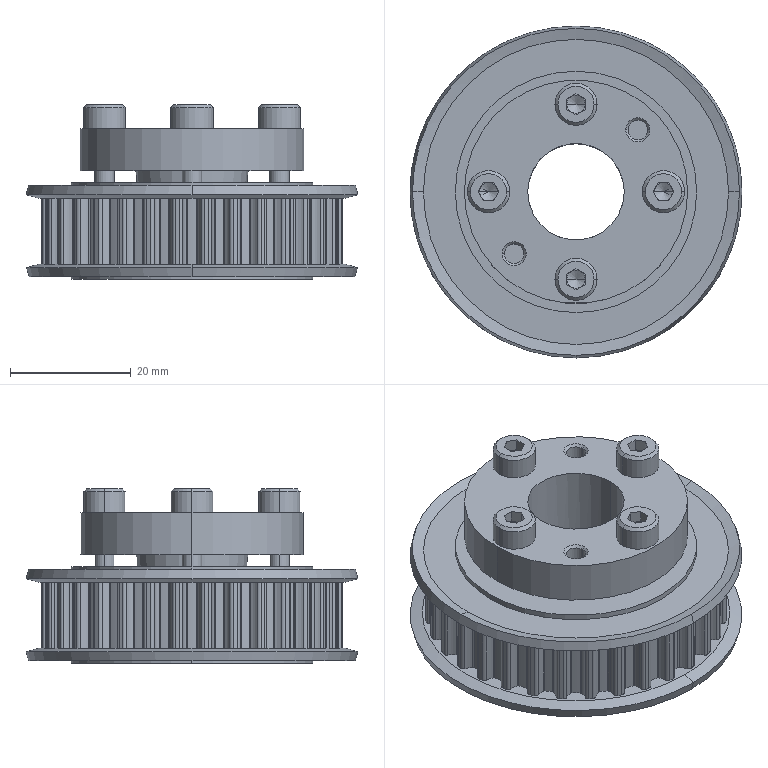Part | STEP file | ECC05-S5M100-32-E-d16 | 1 solid | 413 faces | box 55 x 55 x 29 mm | volume 33207 mm3 | cylinder 313 | plane 60 | cone 40 | commonest cylinder face diameters 1.1 x78 0.5 x74 6.55 x68 46.43 x33 49.97 x32 3.242 x12